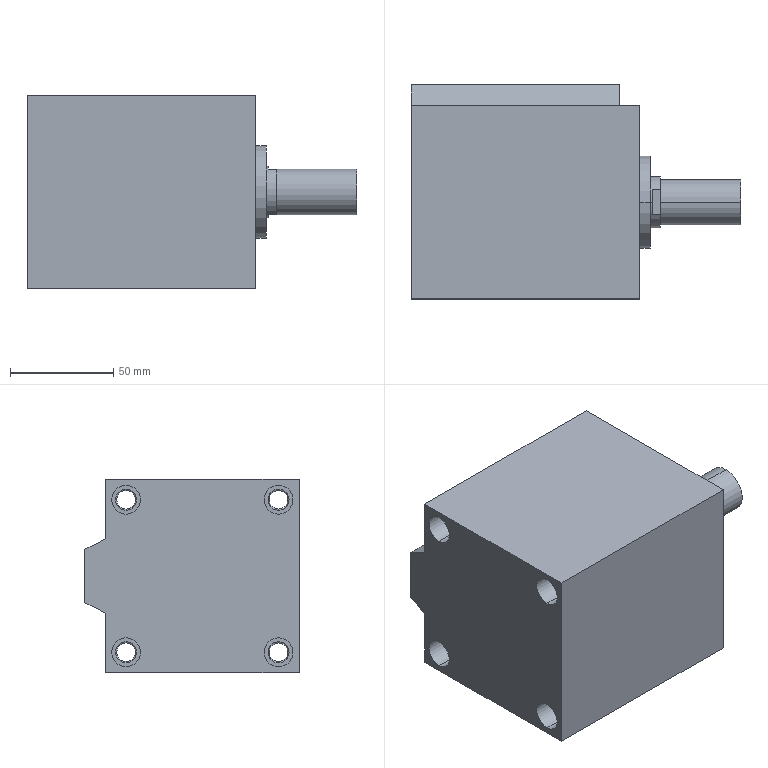Part | STEP file | Cylinder SDA S-80×60 Retract | 2 solids | 89 faces | box 160 x 104 x 94 mm | volume 1037939 mm3 | cylinder 46 | plane 27 | cone 16 | commonest cylinder face diameters 10.2 x16 14 x16 9 x8 22 x2 25 x2 45 x2